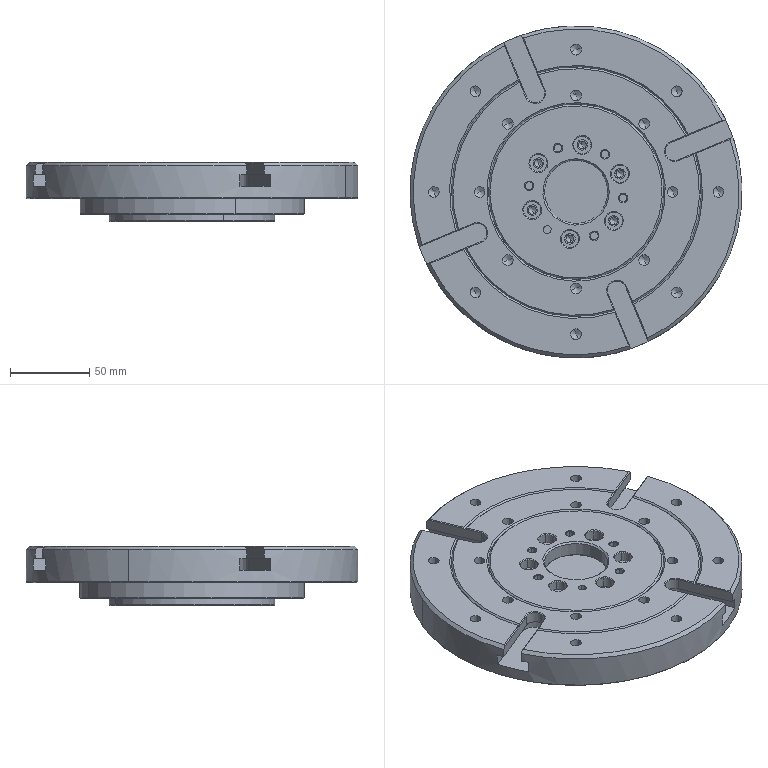NC program | Mastercam | posted with a generic post
Lines 1555 to 3020 of 4738, first 1283 of 1466 lines:
(2.5 DR |TOOL - 2|DIA. OFF. - 2|LEN. - 2|TOOL DIA. - 2.5)
N3174 T2 M6
N3176 G0 G54 G90 X2.703 Y1.185 C90. B-40. S2000 M3
N3178 G43 H2 Z43.769
N3180 G83 G98 Z3.569 R14.769 Q2. F60.
N3182 G80
N3184 M5
N3186 G0 G28 G91 Z0.
N3188 G28 C0. B0.
N3190 M01
N3192 G0 G17 G40 G80 G90 G94 G98
N3194 G0 G28 G91 Z0.
(8 FEMR |TOOL - 1|DIA. OFF. - 1|LEN. - 1|TOOL DIA. - 8.)
N3196 T1 M6
N3198 G0 G54 G90 X1.454 Y13.893 C180. B-90. S3500 M3
N3200 G43 H1 Z50.
N3202 Z10.
N3204 G1 Z-3.75 F2000.
N3206 X1.536 Y13.843
N3208 X2.999 Y12.958 Z-3.92
N3210 G3 X3.755 Y12.707 Z-4. I.932 J1.54
N3212 X4.966 Y12.647 I1.211 J12.296
N3214 G2 X5.74 Y12.587 I-.045 J-5.565
N3216 G3 X9.078 Y12.475 I3.338 J49.866
N3218 X9.394 Y12.476 J49.978
N3220 X13.499 Y12.467 I4.105 J956.23
N3222 X14.175 Y12.468 J956.239
N3224 G1 X14.457 Y12.467
N3226 X14.604
N3228 G3 X15.163 Y12.471 J42.104
N3230 X16.489 Y12.963 I-1.723 J6.677
N3232 X18.866 Y14.132 I-21.079 J45.851
N3234 G2 X20.438 Y14.484 I1.572 J-3.33
N3236 X21.689 Y14.266 J-3.682
N3238 X24.044 Y12.464 I-1.675 J-4.628
N3240 X25.208 Y9.699 I-6.029 J-4.167
N3242 X25.542 Y6.601 I-17.881 J-3.495
N3244 X25.604 Y1.388 I-218.337 J-5.213
N3246 X25.601 Y.258 I-218.399
N3248 G1 X25.602 Y-.025
N3250 Y-14.049
N3252 G3 X25.673 Y-16.053 I270.384 J8.523
N3254 G1 X25.683 Y-16.335
N3256 G2 X25.795 Y-19.773 I-209.226 J-8.554
N3258 G3 X26.006 Y-20.54 Z-3.92 I1.798 J.082
N3260 G1 X26.814 Y-22.049 Z-3.75
N3262 X26.859 Y-22.133
N3264 G3 X27.449 Y-22.486 I.59 J.316 F9500.
N3266 X28.118 Y-21.824 J.669
N3268 G1 X28.37 Y4.863
N3270 G3 X28.371 Y4.981 I-12.406 J.118
N3272 X22.972 Y15.218 I-12.407
N3274 X20.906 Y16.107 I-3.298 J-4.818
N3276 G1 X7.055 Y19.097
N3278 G3 X6.192 Y19.189 I-.863 J-3.995
N3280 X2.105 Y15.102 J-4.087
N3282 X2.832 Y13.657 I1.801
N3284 X3.074 Y13.506 Z-3.778 I1.074 J1.445 F2000.
N3286 G1 X4.337 Y12.847 Z-3.92
N3288 G3 X5.107 Y12.645 Z-4. I.832 J1.597
N3290 G2 X6.225 Y12.459 I-.197 J-4.652
N3292 G3 X8.443 Y12.248 I2.486 J14.339
N3294 X12.696 Y12.192 I4.253 J160.174
N3296 X14.346 Y12.2 J160.23
N3298 X16.077 Y12.589 I-.358 J5.641
N3300 X17.718 Y13.284 I-7.203 J19.282
N3302 G2 X19.479 Y13.634 I1.761 J-4.255
N3304 X21.713 Y13.056 J-4.605
N3306 X23.998 Y10.742 I-2.807 J-5.057
N3308 X24.944 Y8.013 I-7.805 J-4.235
N3310 X25.262 Y4.7 I-22.477 J-3.822
N3312 X25.326 Y-1.105 I-265.238 J-5.805
N3314 X25.321 Y-2.48 I-265.302
N3316 G1 X25.322 Y-2.763
N3318 Y-6.156
N3320 G3 X25.373 Y-7.595 I850.612 J29.166
N3322 G1 X25.383 Y-7.877
N3324 X25.613 Y-14.369
N3326 G3 X25.816 Y-15.138 Z-3.92 I1.799 J.064
N3328 G1 X26.383 Y-16.223 Z-3.798
N3330 G3 X26.654 Y-16.626 Z-3.75 I1.954 J1.02
N3332 G1 X26.928 Y-16.898 F9500.
N3334 X27.245 Y-17.117
N3336 X27.596 Y-17.279
N3338 X27.969 Y-17.376
N3340 X28.354 Y-17.407
N3342 X28.738 Y-17.37
N3344 X29.11 Y-17.267
N3346 X29.458 Y-17.101
N3348 X29.772 Y-16.876
N3350 X30.041 Y-16.6
N3352 X30.259 Y-16.282
N3354 X30.418 Y-15.93
N3356 X30.513 Y-15.556
N3358 X30.541 Y-15.171
N3360 X30.503 Y-14.787
N3362 X25.774 Y9.864
N3364 G3 X18.575 Y16.065 I-7.512 J-1.441
N3366 G1 X4.557 Y16.64
N3368 G3 X4.494 Y16.641 I-.063 J-1.541
N3370 X2.952 Y15.099 J-1.542
N3372 X3.541 Y13.886 I1.542
N3374 X3.6 Y13.842 Z-3.757 I.953 J1.213 F2000.
N3376 G1 X4.259 Y13.373 Z-3.838
N3378 X4.934 Y12.893 Z-3.92
N3380 G3 X5.669 Y12.587 Z-4. I1.043 J1.467
N3382 G2 X6.631 Y12.308 I-.995 J-5.236
N3384 G3 X8.669 Y12.019 I2.473 J10.128
N3386 X12.328 Y11.924 I3.659 J70.285
N3388 X13.88 Y11.941 J70.38
N3390 X16.465 Y12.517 I-.538 J8.505
N3392 G2 X18.74 Y12.985 I2.275 J-5.296
N3394 G1 X18.814 Y12.984
N3396 G2 X22.488 Y11.375 I-.186 J-5.421
N3398 X24.202 Y8.58 I-5.16 J-5.09
N3400 X24.845 Y5.459 I-12.545 J-4.21
N3402 X25.018 Y1.579 I-47.113 J-4.046
N3404 G3 X25.024 Y1.494 I.8 J.011
N3406 G2 X25.083 Y.577 I-8.061 J-.978
N3408 G3 X25.124 Y-.574 I560.825 J19.172
N3410 G1 X25.134 Y-.857
N3412 X25.334 Y-6.501
N3414 G3 X25.537 Y-7.271 Z-3.92 I1.799 J.064
N3416 G1 X26.104 Y-8.356 Z-3.798
N3418 G3 X26.375 Y-8.759 Z-3.75 I1.95 J1.018
N3420 X28.054 Y-9.538 I1.679 J1.421 F9500.
N3422 X30.254 Y-7.338 J2.2
N3424 X30.16 Y-6.703 I-2.2
N3426 G1 X25.393 Y9.117
N3428 G3 X19.127 Y14.282 I-6.999 J-2.109
N3430 G1 X5.063 Y15.7
N3432 G3 X4.959 Y15.705 I-.104 J-1.035
N3434 X3.919 Y14.665 J-1.04
N3436 X4.143 Y14.019 I1.04
N3438 X4.267 Y13.889 Z-3.768 I.816 J.646 F2000.
N3440 G1 X4.869 Y13.352 Z-3.848
N3442 X5.41 Y12.87 Z-3.92
N3444 G3 X6.106 Y12.485 Z-4. I1.197 J1.344
N3446 G2 X6.856 Y12.192 I-1.364 J-4.584
N3448 G3 X8.413 Y11.847 I2.118 J5.887
N3450 X12.118 Y11.664 I3.705 J37.376
N3452 X13.664 Y11.696 J37.559
N3454 X16.029 Y12.145 I-.762 J10.463
N3456 G2 X17.937 Y12.445 I1.908 J-5.914
N3458 X18.957 Y12.361 J-6.214
N3460 X22.448 Y10.315 I-1.092 J-5.866
N3462 X23.931 Y7.613 I-6.2 J-5.159
N3464 X24.561 Y4.391 I-13.959 J-4.406
N3466 X24.649 Y3.221 I-30.123 J-2.849
N3468 G3 X24.687 Y3.022 I.799 J.048
N3470 G2 X25.063 Y1.086 I-7.724 J-2.506
N3472 G3 X25.293 Y.324 Z-3.92 I1.796 J.126
N3474 G1 X25.83 Y-.621 Z-3.812
N3476 G3 X26.221 Y-1.103 Z-3.75 I1.63 J.925
N3478 X27.46 Y-1.571 I1.239 J1.407 F9500.
N3480 X29.335 Y.304 J1.875
N3482 X29.195 Y1.013 I-1.875
N3484 G1 X27.039 Y6.293
N3486 G3 X17.532 Y14.228 I-12.24 J-5.
N3488 G1 X6.77 Y16.502
N3490 G3 X6.395 Y16.541 I-.375 J-1.778
N3492 X4.578 Y14.724 J-1.817
N3494 X4.666 Y14.164 I1.817
N3496 X5.096 Y13.454 Z-3.833 I1.729 J.56 F2000.
N3498 G1 X5.202 Y13.345 Z-3.848
N3500 X5.706 Y12.83 Z-3.92
N3502 G3 X6.375 Y12.398 Z-4. I1.287 J1.258
N3504 G2 X7.183 Y12.014 I-1.624 J-4.465
N3506 G3 X8.7 Y11.63 I2.198 J5.488
N3508 X12.028 Y11.414 I3.328 J25.547
N3510 X13.548 Y11.459 J25.763
N3512 X15.664 Y11.804 I-1.215 J14.101
N3514 G2 X17.208 Y11.979 I1.544 J-6.717
N3516 X18.712 Y11.813 J-6.892
N3518 X22.345 Y9.371 I-1.558 J-6.241
N3520 X23.773 Y6.367 I-7.291 J-5.309
N3522 X24.191 Y4.296 I-16.512 J-4.413
N3524 G3 X24.262 Y4.075 I.79 J.129
N3526 G2 X24.768 Y2.758 I-7.299 J-3.559
N3528 G3 X25.151 Y2.061 Z-3.92 I1.73 J.497
N3530 G1 X25.744 Y1.393 Z-3.831
N3532 G3 X26.396 Y.909 Z-3.75 I1.473 J1.307
N3534 X27.217 Y.73 I.821 J1.791 F9500.
N3536 X29.187 Y2.7 J1.97
N3538 X28.714 Y3.982 I-1.97
N3540 G1 X22.582 Y11.138
N3542 G3 X19.9 Y12.723 I-3.668 J-3.144
N3544 G1 X6.151 Y15.59
N3546 G3 X5.929 Y15.613 I-.222 J-1.064
N3548 X4.842 Y14.526 J-1.087
N3550 X4.931 Y14.099 I1.087
N3552 X5.102 Y13.822 Z-3.783 I.998 J.427 F2000.
N3554 G1 X5.532 Y13.318 Z-3.848
N3556 X5.999 Y12.768 Z-3.92
N3558 G3 X6.636 Y12.291 Z-4. I1.371 J1.167
N3560 G2 X7.411 Y11.859 I-1.999 J-4.493
N3562 G3 X8.842 Y11.432 I2.197 J4.747
N3564 X11.972 Y11.173 I3.13 J18.763
N3566 X13.99 Y11.28 J19.022
N3568 G2 X15.755 Y11.523 I13.678 J-92.651
N3570 X16.537 Y11.567 I.782 J-6.904
N3572 X19.336 Y10.979 J-6.948
N3574 X22.392 Y8.215 I-3.016 J-6.405
N3576 X23.453 Y5.759 I-8.444 J-5.106
N3578 G3 X23.606 Y5.253 I226.126 J68.017
N3580 X23.707 Y5.039 I.765 J.232
N3582 G2 X24.388 Y3.804 I-6.744 J-4.523
N3584 G3 X24.863 Y3.166 Z-3.92 I1.646 J.729
N3586 G1 X25.541 Y2.585 Z-3.831
N3588 G3 X26.259 Y2.206 Z-3.75 I1.197 J1.397
N3590 X26.738 Y2.143 I.479 J1.776 F9500.
N3592 X28.577 Y3.982 J1.839
N3594 X27.976 Y5.342 I-1.839
N3596 G1 X22.034 Y10.755
N3598 G3 X16.759 Y13.439 I-7.522 J-8.258
N3600 G1 X6.639 Y15.517
N3602 G3 X6.412 Y15.54 I-.227 J-1.103
N3604 X5.286 Y14.414 J-1.126
N3606 X5.331 Y14.098 I1.126
N3608 X5.506 Y13.744 Z-3.789 I1.081 J.316 F2000.
N3610 G1 X5.859 Y13.268 Z-3.848
N3612 X6.287 Y12.687 Z-3.92
N3614 G3 X6.89 Y12.168 Z-4. I1.448 J1.07
N3616 G2 X7.554 Y11.737 I-2.599 J-4.735
N3618 G3 X8.839 Y11.267 I2.097 J3.741
N3620 X12.112 Y10.943 I3.273 J16.349
N3622 X14.151 Y11.068 J16.673
N3624 G2 X15.789 Y11.186 I1.638 J-11.308
N3626 X16.426 Y11.168 J-11.426
N3628 X21.682 Y8.233 I-.451 J-6.98
N3630 X22.85 Y6.161 I-9.534 J-6.742
N3632 G3 X22.978 Y5.971 I.721 J.347
N3634 G2 X23.831 Y4.848 I-6.015 J-5.455
N3636 G3 X24.394 Y4.285 Z-3.92 I1.523 J.96
N3638 G1 X25.15 Y3.809 Z-3.831
N3640 G3 X25.914 Y3.538 Z-3.75 I.987 J1.568
N3642 X26.137 Y3.525 I.223 J1.839 F9500.
N3644 X27.989 Y5.377 J1.852
N3646 X27.186 Y6.905 I-1.852
N3648 X26.575 Y7.315 I-9.088 J-12.889
N3650 G1 X13.472 Y15.434
N3652 G3 X9.697 Y16.509 I-3.775 J-6.094
N3654 X6.954 Y15.963 J-7.169
N3656 X5.828 Y14.279 I.697 J-1.684
N3658 X5.837 Y14.11 I1.823
N3660 X6.114 Y13.3 Z-3.836 I1.814 J.169 F2000.
N3662 G1 X6.181 Y13.195 Z-3.848
N3664 X6.569 Y12.587 Z-3.92
N3666 G3 X7.135 Y12.027 Z-4. I1.518 J.967
N3668 G2 X7.777 Y11.551 I-3.714 J-5.686
N3670 G3 X9.26 Y11.007 I2.386 J4.207
N3672 X12.192 Y10.716 I2.932 J14.633
N3674 X13.343 Y10.76 J14.924
N3676 G2 X15.207 Y10.839 I1.864 J-22.091
N3678 X15.521 Y10.836 J-22.17
N3680 X21.098 Y8.077 I-.169 J-7.357
N3682 X21.903 Y7.002 I-14.034 J-11.337
N3684 G3 X22.052 Y6.844 I.65 J.465
N3686 G2 X23.252 Y5.652 I-5.089 J-6.328
N3688 G3 X24.647 Y4.99 Z-3.841 I1.395 J1.139
N3690 X25.526 Y5.22 Z-3.75 J1.801
N3692 X26.447 Y6.791 I-.879 J1.571 F9500.
N3694 X25.319 Y8.46 I-1.8
N3696 G1 X9.097 Y14.997
N3698 G3 X8.424 Y15.128 I-.673 J-1.669
N3700 X6.805 Y14.113 J-1.8
N3702 X6.625 Y13.328 Z-3.831 I1.619 J-.785 F2000.
N3704 X7.369 Y11.869 Z-4. I1.799
N3706 G2 X7.882 Y11.43 I-2.403 J-3.322
N3708 G3 X9.237 Y10.847 I2.294 J3.472
N3710 X12.177 Y10.495 I2.94 J12.106
N3712 X12.501 Y10.5 J12.458
N3714 G2 X14.595 Y10.53 I2.274 J-83.72
N3716 X17.931 Y9.823 I-.062 J-8.513
N3718 X20.355 Y8.134 I-3.495 J-7.598
N3720 X20.767 Y7.727 I-21.673 J-22.353
N3722 G3 X20.94 Y7.595 I.565 J.566
N3724 G2 X22.321 Y6.618 I-3.977 J-7.079
N3726 G3 X23.508 Y6.171 Z-3.871 I1.187 J1.353
N3728 X24.634 Y6.566 Z-3.75 J1.8
N3730 X25.309 Y7.971 I-1.126 J1.405 F9500.
N3732 X24.098 Y9.671 I-1.801
N3734 G1 X9.302 Y14.806
N3736 G3 X8.712 Y14.905 I-.59 J-1.7
N3738 G1 X8.396 Y14.878
N3740 X8.091 Y14.795
N3742 X7.804 Y14.66
N3744 X7.546 Y14.476
N3746 X7.323 Y14.251
N3748 X7.144 Y13.989
N3750 G3 X6.911 Y13.106 Z-3.842 I1.569 J-.884 F2000.
N3752 X7.569 Y11.715 Z-4. I1.801
N3754 G2 X8.049 Y11.265 I-2.63 J-3.289
N3756 G3 X9.327 Y10.665 I2.235 J3.099
N3758 X12.067 Y10.283 I2.867 J10.53
N3760 G2 X14.481 Y10.216 I-.353 J-56.207
N3762 X19.271 Y8.443 I-.541 J-8.821
N3764 G1 X19.517 Y8.267
N3766 X19.54 Y8.251
N3768 G3 X19.733 Y8.149 I.465 J.65
N3770 G2 X21.254 Y7.41 I-2.77 J-7.633
N3772 G3 X22.205 Y7.138 Z-3.9 I.951 J1.528
N3774 X23.545 Y7.736 Z-3.75 J1.8
N3776 X24.005 Y8.938 I-1.34 J1.202 F9500.
N3778 X22.725 Y10.661 I-1.8
N3780 G1 X9.404 Y14.682
N3782 G3 X8.884 Y14.759 I-.52 J-1.723
N3784 X7.351 Y13.902 J-1.8
N3786 X7.084 Y12.959 Z-3.849 I1.533 J-.943 F2000.
N3788 X7.689 Y11.613 Z-4. I1.8
N3790 G2 X7.99 Y11.316 I-2.723 J-3.066
N3792 G1 X7.992 Y11.314
N3794 X7.995 Y11.31
N3796 G3 X8.798 Y10.726 I1.622 J1.386
N3798 X10.98 Y10.155 I2.928 J6.74
N3800 X13.31 Y9.995 I3.425 J32.695
N3802 G2 X16.393 Y9.435 I-.433 J-11.153
N3804 X18.343 Y8.553 I-4.525 J-12.595
N3806 G3 X18.554 Y8.479 I.367 J.71
N3808 G2 X20.169 Y7.977 I-1.591 J-7.963
N3810 G3 X20.879 Y7.831 Z-3.927 I.71 J1.653
N3812 X22.384 Y8.643 Z-3.75 J1.799
N3814 X22.679 Y9.63 I-1.505 J.987 F9500.
N3816 X21.332 Y11.372 I-1.8
N3818 G1 X9.638 Y14.413
N3820 G3 X9.185 Y14.471 I-.453 J-1.742
N3822 X7.723 Y13.72 J-1.8
N3824 X7.386 Y12.671 Z-3.861 I1.462 J-1.049 F2000.
N3826 X7.898 Y11.413 Z-4. I1.799
N3828 G2 X7.99 Y11.316 I-2.932 J-2.866
N3830 G1 X7.992 Y11.314
N3832 X7.995 Y11.31
N3834 G3 X8.723 Y10.665 I2.442 J2.023
N3836 X10.486 Y10.047 I2.673 J4.799
N3838 X12.658 Y9.781 I3.5 J19.595
N3840 G2 X15.849 Y9.19 I-1.084 J-14.764
N3842 X17.263 Y8.67 I-7.137 J-21.584
N3844 G3 X17.497 Y8.618 I.287 J.747
N3846 G2 X18.891 Y8.404 I-.534 J-8.102
N3848 G3 X19.318 Y8.353 Z-3.957 I.427 J1.748
N3850 X20.966 Y9.428 Z-3.75 J1.799
N3852 X21.118 Y10.152 I-1.648 J.724 F9500.
N3854 X19.724 Y11.906 I-1.8
N3856 G1 X9.801 Y14.202
N3858 G3 X9.395 Y14.248 I-.406 J-1.754
N3860 X7.947 Y13.517 J-1.8
N3862 X7.595 Y12.448 Z-3.864 I1.448 J-1.069 F2000.
N3864 X8.091 Y11.207 Z-4. I1.8
N3866 X8.88 Y10.492 I5.047 J4.767
N3868 X10.373 Y9.898 I2.526 J4.18
N3870 X12.528 Y9.541 I4.331 J19.466
N3872 G2 X16.329 Y8.667 I-2.473 J-19.447
N3874 G3 X16.675 Y8.629 I.346 J1.544
N3876 X16.83 Y8.636 J1.582
N3878 G2 X16.932 Y8.637 I.102 J-8.612
N3880 X17.809 Y8.592 J-8.613
N3882 G3 X17.996 Y8.582 Z-3.981 I.187 J1.79
N3884 X19.727 Y9.887 Z-3.75 J1.8
N3886 X19.796 Y10.382 I-1.731 J.495 F9500.
N3888 X18.372 Y12.142 I-1.8
N3890 G1 X10.068 Y13.916
N3892 G3 X9.692 Y13.956 I-.376 J-1.76
N3894 X8.178 Y13.129 J-1.8
N3896 X7.892 Y12.156 Z-3.852 I1.514 J-.973 F2000.
N3898 X8.471 Y10.834 Z-4. I1.8
N3900 X9.288 Y10.179 I4.836 J5.203
N3902 X10.908 Y9.598 I2.725 J5.045
N3904 X13.022 Y9.189 I10.407 J48.173
N3906 G2 X15.252 Y8.66 I-7.184 J-35.253
N3908 G3 X15.574 Y8.629 I.322 J1.635
N3910 X15.73 Y8.636 J1.666
N3912 G1 X16.012
N3914 X16.963
N3916 G3 X18.736 Y10.123 Z-3.75 J1.8
N3918 X18.763 Y10.436 I-1.773 J.313 F9500.
N3920 X17.332 Y12.198 I-1.8
N3922 G1 X10.362 Y13.656
N3924 G3 X9.993 Y13.694 I-.369 J-1.761
N3926 X8.422 Y12.773 J-1.799
N3928 X8.193 Y11.895 Z-3.841 I1.571 J-.878 F2000.
N3930 X8.855 Y10.5 Z-4. I1.8
N3932 X10.009 Y9.739 I3.789 J4.491
N3934 X11.797 Y9.196 I3.7 J8.968
N3936 G2 X14.084 Y8.658 I-31.039 J-136.941
N3938 G3 X14.395 Y8.629 I.311 J1.681
N3940 X14.55 Y8.636 J1.71
N3942 G1 X14.833
N3944 X15.68
N3946 G3 X17.453 Y10.123 Z-3.75 J1.8
N3948 X17.48 Y10.436 I-1.773 J.313 F9500.
N3950 X16.072 Y12.193 I-1.8
N3952 G1 X10.737 Y13.384
N3954 G3 X10.345 Y13.427 I-.392 J-1.757
N3956 X8.717 Y12.396 J-1.8
N3958 X8.545 Y11.627 Z-3.829 I1.628 J-.769 F2000.
N3960 X9.305 Y10.158 Z-4. I1.8
N3962 X11.962 Y8.942 I4.385 J6.073
N3964 X13.871 Y8.636 I1.909 J5.802
N3966 X13.968 Y8.637 J6.108
N3968 X14.371 Y8.635 I.403 J47.108
N3970 X14.654 Y8.636 J47.11
N3972 X16.426 Y10.123 Z-3.75 J1.8
N3974 X16.453 Y10.436 I-1.772 J.313 F9500.
N3976 X15.025 Y12.197 I-1.799
N3978 G1 X11.414 Y12.958
N3980 G3 X11.043 Y12.997 I-.371 J-1.761
N3982 X9.331 Y11.754 J-1.8
N3984 X9.243 Y11.197 Z-3.806 I1.712 J-.557 F2000.
N3986 X10.197 Y9.608 Z-4. I1.8
N3988 X13.005 Y8.707 I3.892 J7.308
N3990 X13.241 Y8.691 Z-3.976 I.236 J1.785
N3992 X13.798 Y8.78 Z-3.92 J1.801
N3994 G1 X15.425 Y9.31 Z-3.75
N3996 X15.518 Y9.34 F9500.
N3998 G0 Z50.
N4000 C188.2 B-270.
N4002 X-9.439 Y-16.51
N4004 Z43.6
N4006 Z-4.4
N4008 G1 Z-6.15 F2000.
N4010 X-9.068 Y-15.343 Z-6.301
N4012 G3 X-8.983 Y-14.798 Z-6.369 I-1.715 J.545
N4014 X-9.001 Y-14.55 Z-6.4 I-1.8
N4016 G1 X-9.059 Y-14.13
N4018 X-9.24 Y-14.097
N4020 G3 X-9.608 Y-14.091 I-.368 J-12.213
N4022 X-11.178 Y-14.193 J-12.219
N4024 X-18.058 Y-15.1 I33.48 J-280.255
N4026 G1 X-18.337 Y-15.139
N4028 X-18.479 Y-15.159
N4030 X-18.401 Y-15.718
N4032 G3 X-16.684 Y-17.269 Z-6.15 I1.782 J.248
N4034 X-16.619 Y-17.27 I.065 J1.799
N4036 X-16.403 Y-17.257 J1.8
N4038 G1 X-10.572 Y-16.553 F9500.
N4040 G3 X-10.234 Y-16.479 I-.216 J1.787
N4042 X-8.988 Y-14.766 Z-6.375 I-.554 J1.713 F2000.
N4044 X-9.005 Y-14.518 Z-6.4 I-1.8
N4046 G1 X-9.063 Y-14.098
N4048 X-9.067 Y-14.07
N4050 G3 X-9.929 Y-13.952 I-.871 J-3.166
N4052 X-10.158 Y-13.951 I-.229 J-18.866
N4054 X-12.532 Y-14.101 J-18.867
N4056 X-17.794 Y-14.798 I16.531 J-145.076
N4058 X-18.504 Y-14.982 I4.282 J-17.951
N4060 G1 X-18.465 Y-15.262
N4062 X-18.426 Y-15.541
N4064 G3 X-16.708 Y-17.092 Z-6.15 I1.783 J.248
N4066 X-16.643 Y-17.093 I.065 J1.799 F9500.
N4068 X-16.462 Y-17.084 J1.8
N4070 G1 X-10.616 Y-16.494
N4072 G3 X-10.243 Y-16.415 I-.181 J1.791
N4074 X-8.998 Y-14.703 Z-6.375 I-.554 J1.712 F2000.
N4076 X-9.014 Y-14.455 Z-6.4 I-1.799
N4078 G1 X-9.072 Y-14.035
N4080 X-9.077 Y-13.999
N4082 G3 X-9.893 Y-13.819 I-1.028 J-2.716
N4084 X-10.965 Y-13.776 I-1.072 J-13.351
N4086 X-12.342 Y-13.847 J-13.394
N4088 X-17.28 Y-14.461 I6.383 J-71.446
N4090 X-18.526 Y-14.82 I.945 J-5.631
N4092 G1 X-18.488 Y-15.099
N4094 X-18.449 Y-15.379
N4096 G3 X-16.731 Y-16.93 Z-6.15 I1.783 J.248
N4098 X-16.666 Y-16.931 I.065 J1.799 F9500.
N4100 X-16.512 Y-16.924 J1.8
N4102 G1 X-10.653 Y-16.421
N4104 G3 X-10.253 Y-16.34 I-.154 J1.794
N4106 X-9.007 Y-14.627 Z-6.375 I-.554 J1.713 F2000.
N4108 X-9.024 Y-14.379 Z-6.4 I-1.8
N4110 G1 X-9.083 Y-13.96
N4112 X-9.088 Y-13.919
N4114 G3 X-9.872 Y-13.689 I-1.151 J-2.477
N4116 X-11.397 Y-13.583 I-1.525 J-10.966
N4118 X-12.208 Y-13.613 J-11.072
N4120 X-17.025 Y-14.169 I2.722 J-44.733
N4122 X-18.194 Y-14.507 I1.007 J-5.681
N4124 X-18.53 Y-14.796 I.334 J-.727
N4126 X-18.217 Y-14.889 Z-6.368 I.669 J1.671
N4128 G1 X-16.074 Y-15.321 Z-6.15
N4130 X-11.174 Y-16.309 F9500.
N4132 G3 X-10.819 Y-16.344 I.355 J1.764
N4134 X-10.265 Y-16.257 J1.799
N4136 X-9.02 Y-14.545 Z-6.375 I-.554 J1.712 F2000.
N4138 X-9.036 Y-14.297 Z-6.4 I-1.799
N4140 G1 X-9.094 Y-13.877
N4142 X-9.1 Y-13.832
N4144 G3 X-9.856 Y-13.562 I-1.252 J-2.31
N4146 X-11.686 Y-13.385 I-1.83 J-9.396
N4148 X-12.099 Y-13.394 J-9.573
N4150 X-16.8 Y-13.888 I.961 J-31.788
N4152 X-18.032 Y-14.271 I.833 J-4.851
N4154 X-18.467 Y-14.562 I.592 J-1.358
N4156 X-18.547 Y-14.669 I.597 J-.532
N4158 G1 X-18.509 Y-14.949
N4160 G3 X-16.791 Y-16.499 Z-6.15 I1.783 J.249
N4162 X-16.726 Y-16.5 I.065 J1.799 F9500.
N4164 X-16.651 Y-16.499 J1.8
N4166 G1 X-10.757 Y-16.255
N4168 G3 X-10.277 Y-16.17 I-.074 J1.798
N4170 X-9.031 Y-14.457 Z-6.375 I-.554 J1.713 F2000.
N4172 X-9.048 Y-14.209 Z-6.4 I-1.8
N4174 G1 X-9.106 Y-13.789
N4176 X-9.113 Y-13.741
N4178 G3 X-9.841 Y-13.437 I-1.336 J-2.171
N4180 X-11.901 Y-13.186 I-2.06 J-8.338
N4182 X-12.007 Y-13.187 J-8.589
N4184 G1 X-12.053
N4186 G3 X-16.795 Y-13.658 J-24.096
N4188 X-18.217 Y-14.213 I.875 J-4.341
N4190 X-18.552 Y-14.637 I.423 J-.678
N4192 G1 X-18.532 Y-14.641 Z-6.398
N4194 X-16.089 Y-15.137 Z-6.15
N4196 X-11.202 Y-16.129 F9500.
N4198 G3 X-10.844 Y-16.165 I.358 J1.764
N4200 X-10.29 Y-16.078 J1.8
N4202 X-9.044 Y-14.365 Z-6.375 I-.554 J1.713 F2000.
N4204 X-9.061 Y-14.117 Z-6.4 I-1.8
N4206 G1 X-9.119 Y-13.697
N4208 X-9.126 Y-13.647
N4210 G3 X-9.981 Y-13.264 I-1.521 J-2.254
N4212 X-12.152 Y-12.98 I-2.2 J-8.364
N4214 X-12.545 Y-12.976 I-.393 J-20.044
N4216 X-16.596 Y-13.39 J-20.048
N4218 X-18.072 Y-13.959 I.979 J-4.739
N4220 X-18.48 Y-14.296 I.711 J-1.272
N4222 X-18.575 Y-14.471 I.649 J-.468
N4224 X-18.515 Y-14.485 Z-6.394 I.433 J1.747
N4226 G1 X-16.117 Y-14.994 Z-6.15
N4228 X-11.231 Y-16.031 F9500.
N4230 G3 X-10.857 Y-16.07 I.374 J1.761
N4232 X-10.303 Y-15.983 J1.8
N4234 X-9.057 Y-14.27 Z-6.375 I-.554 J1.713 F2000.
N4236 X-9.074 Y-14.022 Z-6.4 I-1.8
N4238 G1 X-9.132 Y-13.602
N4240 X-9.14 Y-13.549
N4242 G3 X-9.964 Y-13.135 I-1.587 J-2.132
N4244 X-12.297 Y-12.772 I-2.458 J-8.115
N4246 X-12.885 Y-12.762 I-.588 J-17.135
N4248 X-16.423 Y-13.131 J-17.145
N4250 X-18.092 Y-13.799 I1.062 J-5.071
N4252 X-18.346 Y-13.989 I4.372 J-6.125
N4254 X-18.599 Y-14.298 I.473 J-.645
N4256 G1 X-18.56 Y-14.577
N4258 G3 X-16.843 Y-16.128 Z-6.15 I1.783 J.248
N4260 X-16.777 Y-16.129 I.066 J1.799 F9500.
N4262 G1 X-16.729
N4264 X-10.823 Y-15.971
N4266 G3 X-10.317 Y-15.885 I-.048 J1.799
N4268 X-9.071 Y-14.172 Z-6.375 I-.554 J1.713 F2000.
N4270 X-9.088 Y-13.924 Z-6.4 I-1.8
N4272 G1 X-9.146 Y-13.504
N4274 X-9.154 Y-13.448
N4276 G3 X-9.947 Y-13.006 I-1.598 J-1.939
N4278 X-12.216 Y-12.574 I-2.591 J-7.433
N4280 X-13.118 Y-12.547 I-.902 J-14.902
N4282 X-16.459 Y-12.926 J-14.929
N4284 X-18.124 Y-13.642 I1.204 J-5.089
N4286 X-18.506 Y-14.015 I.724 J-1.125
N4288 X-18.602 Y-14.275 I.691 J-.403
N4290 G2 X-18.408 Y-14.306 Z-6.38 I-.182 J-1.791
N4292 G1 X-16.142 Y-14.789 Z-6.15
N4294 X-11.26 Y-15.831 F9500.
N4296 G3 X-10.885 Y-15.871 I.375 J1.76
N4298 X-10.331 Y-15.784 J1.8
N4300 X-9.085 Y-14.071 Z-6.375 I-.554 J1.713 F2000.
N4302 X-9.102 Y-13.823 Z-6.4 I-1.8
N4304 G1 X-9.16 Y-13.403
N4306 X-9.168 Y-13.344
N4308 G3 X-9.932 Y-12.879 I-1.652 J-1.85
N4310 X-12.139 Y-12.383 I-2.698 J-6.858
N4312 X-13.286 Y-12.333 I-1.147 J-13.236
N4314 X-16.501 Y-12.729 J-13.286
N4316 X-18.118 Y-13.463 I1.26 J-4.919
N4318 X-18.541 Y-13.904 I1.063 J-1.443
N4320 X-18.62 Y-14.144 I.711 J-.368
N4322 X-18.618 Y-14.165 I.795 J.089
N4324 X-16.9 Y-15.716 Z-6.15 I1.783 J.248
N4326 X-16.85 Y-15.717 I.065 J1.799 F9500.
N4328 G1 X-10.914 Y-15.768
N4330 X-10.899
N4332 G3 X-10.345 Y-15.68 J1.8
N4334 X-9.1 Y-13.968 Z-6.375 I-.554 J1.712 F2000.
N4336 X-9.116 Y-13.72 Z-6.4 I-1.799
N4338 G1 X-9.175 Y-13.3
N4340 X-9.183 Y-13.238
N4342 G3 X-10.059 Y-12.687 I-1.857 J-1.979
N4344 X-12.277 Y-12.176 I-2.772 J-6.963
N4346 X-13.409 Y-12.124 I-1.132 J-12.243
N4348 X-16.366 Y-12.484 J-12.295
N4350 X-17.646 Y-12.985 I1.439 J-5.571
N4352 G1 X-17.883 Y-13.138
N4354 G3 X-18.388 Y-13.539 I1.271 J-2.121
N4356 X-18.625 Y-14.026 I.559 J-.573
N4358 X-18.626 Y-14.055 I.8 J-.029
N4360 X-18.618 Y-14.165 I.801
N4362 X-17.578 Y-15.071 Z-6.25 I1.04 J.144
N4364 X-17.277 Y-15.027 Z-6.22 J1.05
N4366 G1 X-16.788 Y-14.881 Z-6.169
N4368 G3 X-16.608 Y-14.808 Z-6.15 I-.3 J1.007
N4370 X-16.07 Y-14.131 I-.48 J.934 F9500.
N4372 X-16.038 Y-13.874 Z-6.176 I-1.018 J.257 F2000.
N4374 X-17.088 Y-12.824 Z-6.34 I-1.05
N4376 X-17.66 Y-12.994 Z-6.4 J-1.05
N4378 G1 X-18.015 Y-13.225
N4380 X-18.261 Y-13.384
N4382 G3 X-18.625 Y-14.055 I.436 J-.671
N4384 X-18.618 Y-14.165 I.8
N4386 X-16.9 Y-15.716 Z-6.15 I1.783 J.248
N4388 X-16.835 Y-15.717 I.065 J1.799 F9500.
N4390 G1 X-16.818
N4392 X-10.897 Y-15.662
N4394 G3 X-10.36 Y-15.575 I-.017 J1.8
N4396 X-9.114 Y-13.862 Z-6.375 I-.554 J1.713 F2000.
N4398 X-9.131 Y-13.614 Z-6.4 I-1.8
N4400 G1 X-9.189 Y-13.194
N4402 X-9.198 Y-13.129
N4404 G3 X-10.04 Y-12.556 I-1.884 J-1.86
N4406 X-12.412 Y-11.968 I-2.904 J-6.64
N4408 X-13.508 Y-11.915 I-1.096 J-11.3
N4410 X-16.428 Y-12.297 J-11.353
N4412 X-17.06 Y-12.604 I.382 J-1.59
N4414 G1 X-17.297 Y-12.758
N4416 X-18.008 Y-13.22
N4418 G3 X-18.486 Y-14.1 Z-6.296 I.572 J-.88
N4420 X-17.616 Y-15.135 Z-6.15 I1.05
N4422 X-17.436 Y-15.151 I.18 J1.035 F9500.
N4424 X-17.411 Y-15.15 J1.051
N4426 G1 X-10.725 Y-14.992
N4428 X-10.403 Y-14.985 Z-6.182 F2000.
N4430 G3 X-9.133 Y-13.685 Z-6.382 I-.03 J1.3
N4432 X-9.146 Y-13.506 Z-6.4 I-1.3
N4434 G1 X-9.204 Y-13.086
N4436 X-9.214 Y-13.018
N4438 G3 X-10.023 Y-12.425 I-1.912 J-1.759
N4440 X-12.335 Y-11.783 I-2.964 J-6.197
N4442 X-13.586 Y-11.711 I-1.251 J-10.843
N4444 X-16.032 Y-11.989 J-10.915
N4446 X-16.513 Y-12.249 I.424 J-1.361
N4448 G1 X-16.749 Y-12.403
N4450 X-17.223 Y-12.71
N4452 G3 X-18.043 Y-14.22 Z-6.222 I.98 J-1.51
N4454 X-17.9 Y-14.923 Z-6.15 I1.8
N4456 X-16.243 Y-16.02 I1.657 J.703 F9500.
N4458 X-16.048 Y-16.009 J1.8
N4460 G1 X-10.75 Y-15.433
N4462 G3 X-10.39 Y-15.356 I-.194 J1.789
N4464 X-9.145 Y-13.644 Z-6.375 I-.554 J1.712 F2000.
N4466 X-9.161 Y-13.396 Z-6.4 I-1.799
N4468 G1 X-9.22 Y-12.976
N4470 X-9.23 Y-12.904
N4472 G3 X-10.006 Y-12.294 I-1.913 J-1.637
N4474 X-12.261 Y-11.603 I-3.013 J-5.808
N4476 X-13.647 Y-11.509 I-1.386 J-10.151
N4478 X-15.562 Y-11.689 J-10.245
N4480 X-16.056 Y-11.952 I.395 J-1.338
N4482 G1 X-16.293 Y-12.106
N4484 X-16.53 Y-12.26
N4486 G3 X-17.349 Y-13.769 Z-6.222 I.981 J-1.509
N4488 X-17.206 Y-14.473 Z-6.15 I1.8
N4490 X-15.549 Y-15.569 I1.657 J.704 F9500.
N4492 X-15.456 Y-15.567 J1.8
N4494 G1 X-10.866 Y-15.329
N4496 G3 X-10.406 Y-15.244 I-.094 J1.798
N4498 X-9.16 Y-13.531 Z-6.375 I-.554 J1.713 F2000.
N4500 X-9.177 Y-13.283 Z-6.4 I-1.8
N4502 G1 X-9.235 Y-12.863
N4504 X-9.246 Y-12.788
N4506 G3 X-9.989 Y-12.164 I-1.913 J-1.525
N4508 X-12.189 Y-11.427 I-3.055 J-5.462
N4510 X-13.675 Y-11.31 I-1.486 J-9.354
N4512 X-15.129 Y-11.422 J-9.471
N4514 X-15.417 Y-11.537 I.148 J-.786
N4516 G1 X-15.654 Y-11.691
N4518 X-16.128 Y-11.999
N4520 G3 X-16.947 Y-13.508 Z-6.222 I.981 J-1.509
N4522 X-16.804 Y-14.212 Z-6.15 I1.8
N4524 X-15.147 Y-15.308 I1.657 J.704 F9500.
N4526 G1 X-15.108
N4528 X-10.936 Y-15.216
N4530 G3 X-10.422 Y-15.129 I-.04 J1.8
N4532 X-9.176 Y-13.416 Z-6.375 I-.554 J1.713 F2000.
N4534 X-9.193 Y-13.168 Z-6.4 I-1.8
N4536 G1 X-9.251 Y-12.749
N4538 X-9.262 Y-12.67
N4540 G3 X-9.974 Y-12.034 I-1.895 J-1.404
N4542 X-12.121 Y-11.254 I-3.086 J-5.15
N4544 X-13.652 Y-11.112 I-1.531 J-8.178
N4546 X-14.754 Y-11.185 J-8.32
N4548 X-15.056 Y-11.303 I.134 J-.789
N4550 G1 X-15.293 Y-11.457
N4552 X-15.767 Y-11.764
N4554 G3 X-16.587 Y-13.274 Z-6.222 I.981 J-1.51
N4556 X-16.443 Y-13.977 Z-6.15 I1.801
N4558 X-14.798 Y-15.074 I1.657 J.703 F9500.
N4560 G1 X-11.004 Y-15.099
N4562 X-10.992
N4564 G3 X-10.438 Y-15.012 J1.8
N4566 X-9.192 Y-13.299 Z-6.375 I-.554 J1.713 F2000.
N4568 X-9.209 Y-13.051 Z-6.4 I-1.8
N4570 G1 X-9.268 Y-12.632
N4572 X-9.279 Y-12.55
N4574 G3 X-10.083 Y-11.823 I-2.103 J-1.519
N4576 X-12.447 Y-11.015 I-3.192 J-5.476
N4578 X-13.586 Y-10.92 I-1.139 J-6.776
N4580 X-14.411 Y-10.97 J-6.871
N4582 X-14.728 Y-11.09 I.119 J-.791
N4584 G1 X-14.965 Y-11.244
N4586 X-15.439 Y-11.551
N4588 G3 X-16.259 Y-13.061 Z-6.222 I.981 J-1.51
N4590 X-16.115 Y-13.764 Z-6.15 I1.801
N4592 X-14.521 Y-14.86 I1.657 J.703 F9500.
N4594 G1 X-11.071 Y-14.979
N4596 G3 X-11.009 Y-14.98 I.062 J1.799
N4598 X-10.455 Y-14.893 J1.8
N4600 X-9.209 Y-13.18 Z-6.375 I-.554 J1.713 F2000.
N4602 X-9.226 Y-12.932 Z-6.4 I-1.8
N4604 G1 X-9.284 Y-12.513
N4606 X-9.296 Y-12.427
N4608 G3 X-10.193 Y-11.609 I-2.165 J-1.474
N4610 X-12.569 Y-10.812 I-3.186 J-5.556
N4612 X-13.467 Y-10.736 I-.898 J-5.279
N4614 X-14.117 Y-10.776 J-5.355
N4616 X-14.428 Y-10.895 I.125 J-.79
N4618 G1 X-14.665 Y-11.049
N4620 X-15.139 Y-11.356
N4622 G3 X-15.959 Y-12.866 Z-6.222 I.981 J-1.51
N4624 X-15.815 Y-13.569 Z-6.15 I1.801
N4626 X-14.269 Y-14.663 I1.657 J.703 F9500.
N4628 G1 X-11.136 Y-14.856
N4630 G3 X-11.025 Y-14.859 I.111 J1.797
N4632 X-10.471 Y-14.772 J1.8
N4634 X-9.225 Y-13.059 Z-6.375 I-.554 J1.713 F2000.
N4636 X-9.243 Y-12.811 Z-6.4 I-1.8
N4638 G1 X-9.301 Y-12.392
N4640 X-9.313 Y-12.302
N4642 G3 X-10.174 Y-11.473 I-2.259 J-1.485
N4644 X-12.857 Y-10.594 I-3.259 J-5.412
N4646 X-13.344 Y-10.566 I-.487 J-4.228
N4648 X-13.822 Y-10.593 J-4.256
N4650 X-14.151 Y-10.715 I.107 J-.793
N4652 G1 X-14.388 Y-10.869
N4654 X-14.625 Y-11.023
N4656 G3 X-15.444 Y-12.532 Z-6.222 I.981 J-1.509
N4658 X-15.301 Y-13.236 Z-6.15 I1.8
N4660 X-13.92 Y-14.311 I1.657 J.704 F9500.
N4662 G1 X-11.319 Y-14.715
N4664 G3 X-11.043 Y-14.736 I.276 J1.779
N4666 X-10.489 Y-14.649 J1.8
N4668 X-9.243 Y-12.936 Z-6.375 I-.554 J1.713 F2000.
N4670 X-9.26 Y-12.688 Z-6.4 I-1.8
N4672 G1 X-9.318 Y-12.268
N4674 X-9.331 Y-12.174
N4676 G3 X-10.283 Y-11.254 I-2.374 J-1.504
N4678 X-13.299 Y-10.413 I-3.016 J-4.986
N4680 X-13.47 Y-10.416 J-5.827
N4682 G1 X-13.546 Y-10.424
N4684 G3 X-13.894 Y-10.548 I.087 J-.795
N4686 G1 X-14.131 Y-10.702
N4688 X-14.368 Y-10.856
N4690 G3 X-15.188 Y-12.366 Z-6.222 I.98 J-1.51
N4692 X-15.045 Y-13.069 Z-6.15 I1.8
N4694 X-13.726 Y-14.134 I1.657 J.703 F9500.
N4696 G1 X-11.398 Y-14.579
N4698 G3 X-11.06 Y-14.611 I.338 J1.768
N4700 X-10.506 Y-14.523 J1.8
N4702 X-9.261 Y-12.811 Z-6.375 I-.554 J1.712 F2000.
N4704 X-9.277 Y-12.563 Z-6.4 I-1.799
N4706 G1 X-9.336 Y-12.143
N4708 X-9.349 Y-12.043
N4710 G3 X-10.264 Y-11.116 I-2.396 J-1.447
N4712 X-13.182 Y-10.259 I-2.918 J-4.54
N4714 G1 X-13.187
N4716 X-13.286 Y-10.267
N4718 G3 X-13.656 Y-10.393 I.066 J-.797
N4720 G1 X-13.893 Y-10.547
N4722 X-14.129 Y-10.701
N4724 G3 X-14.949 Y-12.211 Z-6.222 I.98 J-1.51
N4726 X-14.806 Y-12.914 Z-6.15 I1.8
N4728 X-13.55 Y-13.966 I1.657 J.703 F9500.
N4730 G1 X-11.478 Y-14.438
N4732 G3 X-11.078 Y-14.483 I.4 J1.755
N4734 X-10.524 Y-14.396 J1.8
N4736 X-9.278 Y-12.683 Z-6.375 I-.554 J1.713 F2000.
N4738 X-9.295 Y-12.435 Z-6.4 I-1.8
N4740 G1 X-9.353 Y-12.016
N4742 X-9.368 Y-11.91
N4744 G3 X-10.247 Y-10.976 I-2.433 J-1.41
N4746 X-12.918 Y-10.114 I-2.801 J-4.109
N4748 G1 X-12.928
N4750 G3 X-13.34 Y-10.197 J-1.067
N4752 X-13.908 Y-10.557 I2.384 J-4.387
N4754 X-14.728 Y-12.067 Z-6.222 I.981 J-1.51
N4756 X-14.584 Y-12.77 Z-6.15 I1.801
N4758 X-13.39 Y-13.806 I1.657 J.703 F9500.
N4760 G1 X-11.559 Y-14.293
N4762 G3 X-11.096 Y-14.354 I.463 J1.739
N4764 X-10.542 Y-14.267 J1.8
N4766 X-9.296 Y-12.554 Z-6.375 I-.554 J1.713 F2000.
N4768 X-9.313 Y-12.306 Z-6.4 I-1.8
N4770 G1 X-9.371 Y-11.886
N4772 X-9.387 Y-11.774
N4774 G3 X-10.233 Y-10.836 I-2.37 J-1.286
N4776 X-12.664 Y-9.981 I-2.688 J-3.762
N4778 X-12.713 Y-9.98 I-.049 J-1.124
N4780 X-13.112 Y-10.053 J-1.125
N4782 X-13.7 Y-10.422 I2.008 J-3.85
N4784 X-14.52 Y-11.932 Z-6.222 I.98 J-1.51
N4786 X-14.376 Y-12.635 Z-6.15 I1.8
N4788 X-13.245 Y-13.653 I1.656 J.703 F9500.
N4790 G1 X-11.64 Y-14.144
N4792 G3 X-11.114 Y-14.223 I.526 J1.722
N4794 X-10.56 Y-14.135 J1.801
N4796 X-9.314 Y-12.422 Z-6.375 I-.554 J1.713 F2000.
N4798 X-9.331 Y-12.174 Z-6.4 I-1.8
N4800 G1 X-9.39 Y-11.755
N4802 X-9.406 Y-11.634
N4804 G3 X-10.22 Y-10.694 I-2.322 J-1.188
N4806 X-12.529 Y-9.856 I-2.526 J-3.36
N4808 G1 X-12.621 Y-9.859
N4810 G3 X-13.031 Y-9.988 I.025 J-.8
N4812 G1 X-13.268 Y-10.142
N4814 X-13.505 Y-10.295
N4816 G3 X-14.325 Y-11.805 Z-6.222 I.98 J-1.51
N4818 X-14.181 Y-12.508 Z-6.15 I1.8
N4820 X-13.113 Y-13.506 I1.656 J.703 F9500.
N4822 G1 X-11.721 Y-13.988
N4824 G3 X-11.133 Y-14.087 I.588 J1.701
N4826 X-10.579 Y-13.999 J1.8
N4828 X-9.334 Y-12.287 Z-6.375 I-.554 J1.712 F2000.
N4830 X-9.35 Y-12.038 Z-6.4 I-1.799
N4832 G1 X-9.408 Y-11.619
N4834 X-9.426 Y-11.493
N4836 G3 X-10.206 Y-10.556 I-2.266 J-1.093
N4838 X-12.298 Y-9.74 I-2.399 J-3.06
N4840 X-12.361 Y-9.738 I-.063 J-1.042
N4842 X-12.717 Y-9.8 J-1.044
N4844 X-13.086 Y-10.023 I.668 J-1.522
N4846 G1 X-13.323 Y-10.177
N4848 G3 X-14.143 Y-11.687 Z-6.222 I.981 J-1.51
N4850 X-13.999 Y-12.39 Z-6.15 I1.801
N4852 X-12.993 Y-13.365 I1.657 J.703 F9500.
N4854 G1 X-11.803 Y-13.826
N4856 G3 X-11.152 Y-13.948 I.651 J1.678
N4858 X-10.598 Y-13.861 J1.8
N4860 X-9.352 Y-12.148 Z-6.375 I-.554 J1.713 F2000.
N4862 X-9.369 Y-11.9 Z-6.4 I-1.8
N4864 G1 X-9.428 Y-11.481
N4866 X-9.475 Y-11.281
N4868 G3 X-10.42 Y-10.251 I-2.479 J-1.327
N4870 X-12.176 Y-9.628 I-1.994 J-2.835
N4872 G1 X-12.246 Y-9.629
N4874 G3 X-12.677 Y-9.758 I.005 J-.8
N4876 G1 X-12.914 Y-9.912
N4878 X-13.151 Y-10.065
N4880 G3 X-13.971 Y-11.575 Z-6.222 I.981 J-1.51
N4882 X-13.827 Y-12.278 Z-6.15 I1.801
N4884 X-12.886 Y-13.226 I1.657 J.703 F9500.
N4886 G1 X-11.888 Y-13.66
N4888 G3 X-11.172 Y-13.808 I.716 J1.652
N4890 X-10.618 Y-13.721 J1.8
N4892 X-9.372 Y-12.008 Z-6.375 I-.554 J1.713 F2000.
N4894 X-9.389 Y-11.76 Z-6.4 I-1.8
N4896 G1 X-9.447 Y-11.34
N4898 X-9.493 Y-11.135
N4900 G3 X-10.403 Y-10.115 I-2.395 J-1.219
N4902 X-11.972 Y-9.526 I-1.883 J-2.633
N4904 G1 X-12.059 Y-9.524
N4906 X-12.079
N4908 G3 X-12.515 Y-9.652 J-.799
N4910 G1 X-12.752 Y-9.806
N4912 X-12.989 Y-9.96
N4914 G3 X-13.809 Y-11.47 Z-6.222 I.981 J-1.51
N4916 X-13.665 Y-12.173 Z-6.15 I1.801
N4918 X-12.794 Y-13.089 I1.657 J.703 F9500.
N4920 G1 X-11.977 Y-13.485
N4922 G3 X-11.191 Y-13.666 I.786 J1.619
N4924 X-10.638 Y-13.579 J1.8
N4926 X-9.391 Y-11.866 Z-6.375 I-.553 J1.713 F2000.
N4928 X-9.409 Y-11.618 Z-6.4 I-1.8
N4930 G1 X-9.467 Y-11.198
N4932 X-9.513 Y-10.986
N4934 G3 X-10.504 Y-9.902 I-2.35 J-1.155
N4936 X-11.914 Y-9.425 I-1.572 J-2.325
N4938 G1 X-11.927
N4940 G3 X-12.363 Y-9.554 J-.8
N4942 G1 X-12.6 Y-9.708
N4944 X-12.837 Y-9.861
N4946 G3 X-13.657 Y-11.371 Z-6.222 I.981 J-1.51
N4948 X-13.513 Y-12.074 Z-6.15 I1.801
N4950 X-12.714 Y-12.954 I1.657 J.703 F9500.
N4952 G1 X-12.069 Y-13.303
N4954 G3 X-11.212 Y-13.52 I.857 J1.583
N4956 X-10.658 Y-13.433 J1.8
N4958 X-9.412 Y-11.72 Z-6.375 I-.554 J1.713 F2000.
N4960 X-9.429 Y-11.472 Z-6.4 I-1.8
N4962 G1 X-9.487 Y-11.053
N4964 X-9.532 Y-10.836
N4966 G3 X-10.485 Y-9.773 I-2.283 J-1.09
N4968 X-11.724 Y-9.333 I-1.458 J-2.139
N4970 X-11.767 Y-9.332 I-.043 J-.799
N4972 X-12.087 Y-9.399 J-.8
N4974 X-12.505 Y-9.646 I.81 J-1.848
N4976 G1 X-12.742 Y-9.8
N4978 G3 X-13.562 Y-11.31 Z-6.222 I.98 J-1.51
N4980 X-13.419 Y-12.013 Z-6.15 I1.8
N4982 X-12.553 Y-12.926 I1.657 J.703 F9500.
N4984 G1 X-12.024 Y-13.185
N4986 G3 X-11.233 Y-13.368 I.791 J1.616
N4988 X-10.679 Y-13.281 J1.799
N4990 X-9.434 Y-11.569 Z-6.375 I-.554 J1.712 F2000.
N4992 X-9.45 Y-11.321 Z-6.4 I-1.799
N4994 G1 X-9.508 Y-10.901
N4996 X-9.551 Y-10.689
N4998 G3 X-10.457 Y-9.656 I-2.166 J-.985
N5000 X-11.368 Y-9.273 I-1.45 J-2.179
N5002 X-11.537 Y-9.259 I-.169 J-1.024
N5004 X-11.95 Y-9.345 J-1.038
N5006 X-12.505 Y-9.646 I.67 J-1.897
N5008 X-13.325 Y-11.156 Z-6.222 I.98 J-1.51
N5010 X-13.182 Y-11.859 Z-6.15 I1.8
N5012 X-12.78 Y-12.446 I1.657 J.703 F9500.
N5014 G1 X-12.508 Y-12.71
N5016 G3 X-11.254 Y-13.219 I1.254 J1.29
N5018 X-10.7 Y-13.132 J1.799
N5020 X-9.455 Y-11.42 Z-6.375 I-.554 J1.712 F2000.
N5022 X-9.471 Y-11.172 Z-6.4 I-1.799
N5024 G1 X-9.529 Y-10.752
N5026 X-9.571 Y-10.539
N5028 G3 X-10.549 Y-9.468 I-2.128 J-.963
N5030 X-11.329 Y-9.229 I-.78 J-1.152
N5032 X-11.659 Y-9.268 J-1.391
N5034 X-11.932 Y-9.339 I.347 J-1.905
N5036 X-12.954 Y-10.496 Z-6.239 I.497 J-1.468
N5038 G1 X-13.038 Y-10.906 Z-6.198
N5040 G3 X-13.075 Y-11.268 Z-6.161 I1.763 J-.362
N5042 X-13.071 Y-11.383 Z-6.15 I1.8
N5044 X-11.275 Y-13.068 I1.796 J.115 F9500.
N5046 X-10.721 Y-12.981 J1.8
N5048 X-9.475 Y-11.268 Z-6.375 I-.554 J1.713 F2000.
N5050 X-9.492 Y-11.02 Z-6.4 I-1.8
N5052 G1 X-9.55 Y-10.6
N5054 X-9.59 Y-10.39
N5056 G3 X-11.289 Y-9.233 I-1.699 J-.669
N5058 X-11.531 Y-9.249 J-1.826
N5060 X-13.124 Y-10.928 Z-6.15 I.204 J-1.789
N5062 X-13.127 Y-11.038 I1.797 J-.11 F9500.
N5064 X-13.001 Y-11.699 I1.8
N5066 X-11.295 Y-12.917 I1.706 J.586
N5068 X-10.742 Y-12.83 J1.804
N5070 X-9.496 Y-11.117 Z-6.375 I-.554 J1.713 F2000.
N5072 X-9.513 Y-10.869 Z-6.4 I-1.8
N5074 G1 X-9.571 Y-10.449
N5076 X-9.573 Y-10.433
N5078 G3 X-9.873 Y-9.877 I-1.038 J-.201
N5080 X-10.557 Y-9.39 I-1.439 J-1.296
N5082 X-11.259 Y-9.248 Z-6.328 I-.702 J-1.658
N5084 X-12.522 Y-9.765 Z-6.189 J-1.8
N5086 G1 X-12.802 Y-10.041 Z-6.15
N5088 X-14.699 Y-11.91 F9500.
N5090 G0 Z43.6
N5092 C179.905 B-272.298
N5094 X-25.94 Y-16.16
N5096 Z42.615
N5098 Z-6.385
N5100 G1 Z-7.385 F2000.
N5102 G41 D1 X-25.734 Y-11.164 F1000.
N5104 X-25.066 Y4.999
N5106 G40 X-24.86 Y9.995
N5108 G0 Z42.615
N5110 X-25.69 Y-16.17
N5112 Z-6.385
N5114 G1 Z-7.385 F2000.
N5116 G41 D1 X-25.484 Y-11.174 F1000.
N5118 X-24.816 Y4.989
N5120 G40 X-24.61 Y9.985
N5122 G0 Z42.615
N5124 M5
N5126 G0 G28 G91 Z0.
N5128 G28 C0. B0.
N5130 M01
N5132 G0 G17 G40 G80 G90 G94 G98
N5134 G0 G28 G91 Z0.
(4 FEMR |TOOL - 5|DIA. OFF. - 5|LEN. - 5|TOOL DIA. - 4.)
N5136 T5 M6
N5138 G0 G54 G90 X22.306 Y14.817 C8.2 B-90. S3500 M3
N5140 G43 H5 Z50.
N5142 Z3.1
N5144 G1 Z1.822 F2000.
N5146 G41 D5 X20.981 Y12.697 F500.
N5148 X17.485 Y7.102
N5150 X17.361 Y3.54
N5152 X20.431 Y5.534
N5154 X23.979 Y11.211
N5156 G40 X25.303 Y13.332
N5158 Z1.544 F2000.
N5160 G42 D5 X23.979 Y11.211 F500.
N5162 X20.431 Y5.534
N5164 X17.361 Y3.54
N5166 X17.485 Y7.102
N5168 X20.981 Y12.697
N5170 G40 X22.306 Y14.817
N5172 Z1.266 F2000.
N5174 G41 D5 X20.981 Y12.697 F500.
N5176 X17.485 Y7.102
N5178 X17.361 Y3.54
N5180 X20.431 Y5.534
N5182 X23.979 Y11.211
N5184 G40 X25.303 Y13.332
N5186 Z.988 F2000.
N5188 G42 D5 X23.979 Y11.211 F500.
N5190 X20.431 Y5.534
N5192 X17.361 Y3.54
N5194 X17.485 Y7.102
N5196 X20.981 Y12.697
N5198 G40 X22.306 Y14.817
N5200 Z.71 F2000.
N5202 G41 D5 X20.981 Y12.697 F500.
N5204 X17.485 Y7.102
N5206 X17.361 Y3.54
N5208 X20.431 Y5.534
N5210 X23.979 Y11.211
N5212 G40 X25.303 Y13.332
N5214 Z.432 F2000.
N5216 G42 D5 X23.979 Y11.211 F500.
N5218 X20.431 Y5.534
N5220 X17.361 Y3.54
N5222 X17.485 Y7.102
N5224 X20.981 Y12.697
N5226 G40 X22.306 Y14.817
N5228 Z.154 F2000.
N5230 G41 D5 X20.981 Y12.697 F500.
N5232 X17.485 Y7.102
N5234 X17.361 Y3.54
N5236 X20.431 Y5.534
N5238 X23.979 Y11.211
N5240 G40 X25.303 Y13.332
N5242 Z-.124 F2000.
N5244 G42 D5 X23.979 Y11.211 F500.
N5246 X20.431 Y5.534
N5248 X17.361 Y3.54
N5250 X17.485 Y7.102
N5252 X20.981 Y12.697
N5254 G40 X22.306 Y14.817
N5256 Z-.402 F2000.
N5258 G41 D5 X20.981 Y12.697 F500.
N5260 X17.485 Y7.102
N5262 X17.361 Y3.54
N5264 X20.431 Y5.534
N5266 X23.979 Y11.211
N5268 G40 X25.303 Y13.332
N5270 Z-.68 F2000.
N5272 G42 D5 X23.979 Y11.211 F500.
N5274 X20.431 Y5.534
N5276 X17.361 Y3.54
N5278 X17.485 Y7.102
N5280 X20.981 Y12.697
N5282 G40 X22.306 Y14.817
N5284 G0 Z50.
N5286 M5
N5288 G0 G28 G91 Z0.
N5290 G28 C0. B0.
N5292 M01
N5294 G0 G17 G40 G80 G90 G94 G98
N5296 G0 G28 G91 Z0.
(2 FEMR |TOOL - 6|DIA. OFF. - 6|LEN. - 6|TOOL DIA. - 2.)
N5298 T6 M6
N5300 G0 G54 G90 X17.021 Y5.279 C8.2 B-90. S5000 M3
N5302 G43 H6 Z50.
N5304 Z2.9
N5306 G1 Z1.801 F600.
N5308 G41 D6 X16.521 Y5.297
N5310 X16.518
N5312 G3 X16.418 Y5.2 J-.1
N5314 G1 X16.314 Y2.223
N5316 X15.179 Y.18
N5318 G3 X15.142 Y.039 I.254 J-.141
N5320 X15.433 Y-.252 I.291
N5322 X15.686 Y-.102 J.291
N5324 G1 X16.87 Y2.029
N5326 X19.269 Y3.587
N5328 G3 X19.315 Y3.671 I-.054 J.084
N5330 X19.299 Y3.725 I-.1
N5332 G1 G40 X19.026 Y4.145
N5334 X17.021 Y5.279
N5336 Z1.702
N5338 G41 D6 X16.521 Y5.297
N5340 X16.518
N5342 G3 X16.418 Y5.2 J-.1
N5344 G1 X16.314 Y2.223
N5346 X15.179 Y.18
N5348 G3 X15.142 Y.039 I.254 J-.141
N5350 X15.433 Y-.252 I.291
N5352 X15.686 Y-.102 J.291
N5354 G1 X16.87 Y2.029
N5356 X19.269 Y3.587
N5358 G3 X19.315 Y3.671 I-.054 J.084
N5360 X19.299 Y3.725 I-.1
N5362 G1 G40 X19.026 Y4.145
N5364 X17.021 Y5.279
N5366 Z1.602
N5368 G41 D6 X16.521 Y5.297
N5370 X16.518
N5372 G3 X16.418 Y5.2 J-.1
N5374 G1 X16.314 Y2.223
N5376 X15.179 Y.18
N5378 G3 X15.142 Y.039 I.254 J-.141
N5380 X15.433 Y-.252 I.291
N5382 X15.686 Y-.102 J.291
N5384 G1 X16.87 Y2.029
N5386 X19.269 Y3.587
N5388 G3 X19.315 Y3.671 I-.054 J.084
N5390 X19.299 Y3.725 I-.1
N5392 G1 G40 X19.026 Y4.145
N5394 X17.021 Y5.279
N5396 Z1.503
N5398 G41 D6 X16.521 Y5.297
N5400 X16.518
N5402 G3 X16.418 Y5.2 J-.1
N5404 G1 X16.314 Y2.223
N5406 X15.179 Y.18
N5408 G3 X15.142 Y.039 I.254 J-.141
N5410 X15.433 Y-.252 I.291
N5412 X15.686 Y-.102 J.291
N5414 G1 X16.87 Y2.029
N5416 X19.269 Y3.587
N5418 G3 X19.315 Y3.671 I-.054 J.084
N5420 X19.299 Y3.725 I-.1
N5422 G1 G40 X19.026 Y4.145
N5424 X17.021 Y5.279
N5426 Z1.404
N5428 G41 D6 X16.521 Y5.297
N5430 X16.518
N5432 G3 X16.418 Y5.2 J-.1
N5434 G1 X16.314 Y2.223
N5436 X15.179 Y.18
N5438 G3 X15.142 Y.039 I.254 J-.141
N5440 X15.433 Y-.252 I.291
N5442 X15.686 Y-.102 J.291
N5444 G1 X16.87 Y2.029
N5446 X19.269 Y3.587
N5448 G3 X19.315 Y3.671 I-.054 J.084
N5450 X19.299 Y3.725 I-.1
N5452 G1 G40 X19.026 Y4.145
N5454 X17.021 Y5.279
N5456 Z1.305
N5458 G41 D6 X16.521 Y5.297
N5460 X16.518
N5462 G3 X16.418 Y5.2 J-.1
N5464 G1 X16.314 Y2.223
N5466 X15.179 Y.18
N5468 G3 X15.142 Y.039 I.254 J-.141
N5470 X15.433 Y-.252 I.291
N5472 X15.686 Y-.102 J.291
N5474 G1 X16.87 Y2.029
N5476 X19.269 Y3.587
N5478 G3 X19.315 Y3.671 I-.054 J.084
N5480 X19.299 Y3.725 I-.1
N5482 G1 G40 X19.026 Y4.145
N5484 X17.021 Y5.279
N5486 Z1.205
N5488 G41 D6 X16.521 Y5.297
N5490 X16.518
N5492 G3 X16.418 Y5.2 J-.1
N5494 G1 X16.314 Y2.223
N5496 X15.179 Y.18
N5498 G3 X15.142 Y.039 I.254 J-.141
N5500 X15.433 Y-.252 I.291
N5502 X15.686 Y-.102 J.291
N5504 G1 X16.87 Y2.029
N5506 X19.269 Y3.587
N5508 G3 X19.315 Y3.671 I-.054 J.084
N5510 X19.299 Y3.725 I-.1
N5512 G1 G40 X19.026 Y4.145
N5514 X17.021 Y5.279
N5516 Z1.106
N5518 G41 D6 X16.521 Y5.297
N5520 X16.518
N5522 G3 X16.418 Y5.2 J-.1
N5524 G1 X16.314 Y2.223
N5526 X15.179 Y.18
N5528 G3 X15.142 Y.039 I.254 J-.141
N5530 X15.433 Y-.252 I.291
N5532 X15.686 Y-.102 J.291
N5534 G1 X16.87 Y2.029
N5536 X19.269 Y3.587
N5538 G3 X19.315 Y3.671 I-.054 J.084
N5540 X19.299 Y3.725 I-.1
N5542 G1 G40 X19.026 Y4.145
N5544 X17.021 Y5.279
N5546 Z1.007
N5548 G41 D6 X16.521 Y5.297
N5550 X16.518
N5552 G3 X16.418 Y5.2 J-.1
N5554 G1 X16.314 Y2.223
N5556 X15.179 Y.18
N5558 G3 X15.142 Y.039 I.254 J-.141
N5560 X15.433 Y-.252 I.291
N5562 X15.686 Y-.102 J.291
N5564 G1 X16.87 Y2.029
N5566 X19.269 Y3.587
N5568 G3 X19.315 Y3.671 I-.054 J.084
N5570 X19.299 Y3.725 I-.1
N5572 G1 G40 X19.026 Y4.145
N5574 X17.021 Y5.279
N5576 Z.908
N5578 G41 D6 X16.521 Y5.297
N5580 X16.518
N5582 G3 X16.418 Y5.2 J-.1
N5584 G1 X16.314 Y2.223
N5586 X15.179 Y.18
N5588 G3 X15.142 Y.039 I.254 J-.141
N5590 X15.433 Y-.252 I.291
N5592 X15.686 Y-.102 J.291
N5594 G1 X16.87 Y2.029
N5596 X19.269 Y3.587
N5598 G3 X19.315 Y3.671 I-.054 J.084
N5600 X19.299 Y3.725 I-.1
N5602 G1 G40 X19.026 Y4.145
N5604 X17.021 Y5.279
N5606 Z.808
N5608 G41 D6 X16.521 Y5.297
N5610 X16.518
N5612 G3 X16.418 Y5.2 J-.1
N5614 G1 X16.314 Y2.223
N5616 X15.179 Y.18
N5618 G3 X15.142 Y.039 I.254 J-.141
N5620 X15.433 Y-.252 I.291
N5622 X15.686 Y-.102 J.291
N5624 G1 X16.87 Y2.029
N5626 X19.269 Y3.587
N5628 G3 X19.315 Y3.671 I-.054 J.084
N5630 X19.299 Y3.725 I-.1
N5632 G1 G40 X19.026 Y4.145
N5634 X17.021 Y5.279
N5636 Z.709
N5638 G41 D6 X16.521 Y5.297
N5640 X16.518
N5642 G3 X16.418 Y5.2 J-.1
N5644 G1 X16.314 Y2.223
N5646 X15.179 Y.18
N5648 G3 X15.142 Y.039 I.254 J-.141
N5650 X15.433 Y-.252 I.291
N5652 X15.686 Y-.102 J.291
N5654 G1 X16.87 Y2.029
N5656 X19.269 Y3.587
N5658 G3 X19.315 Y3.671 I-.054 J.084
N5660 X19.299 Y3.725 I-.1
N5662 G1 G40 X19.026 Y4.145
N5664 X17.021 Y5.279
N5666 Z.61
N5668 G41 D6 X16.521 Y5.297
N5670 X16.518
N5672 G3 X16.418 Y5.2 J-.1
N5674 G1 X16.314 Y2.223
N5676 X15.179 Y.18
N5678 G3 X15.142 Y.039 I.254 J-.141
N5680 X15.433 Y-.252 I.291
N5682 X15.686 Y-.102 J.291
N5684 G1 X16.87 Y2.029
N5686 X19.269 Y3.587
N5688 G3 X19.315 Y3.671 I-.054 J.084
N5690 X19.299 Y3.725 I-.1
N5692 G1 G40 X19.026 Y4.145
N5694 X17.021 Y5.279
N5696 Z.511
N5698 G41 D6 X16.521 Y5.297
N5700 X16.518
N5702 G3 X16.418 Y5.2 J-.1
N5704 G1 X16.314 Y2.223
N5706 X15.179 Y.18
N5708 G3 X15.142 Y.039 I.254 J-.141
N5710 X15.433 Y-.252 I.291
N5712 X15.686 Y-.102 J.291
N5714 G1 X16.87 Y2.029
N5716 X19.269 Y3.587
N5718 G3 X19.315 Y3.671 I-.054 J.084
N5720 X19.299 Y3.725 I-.1
N5722 G1 G40 X19.026 Y4.145
N5724 X17.021 Y5.279
N5726 Z.412
N5728 G41 D6 X16.521 Y5.297
N5730 X16.518